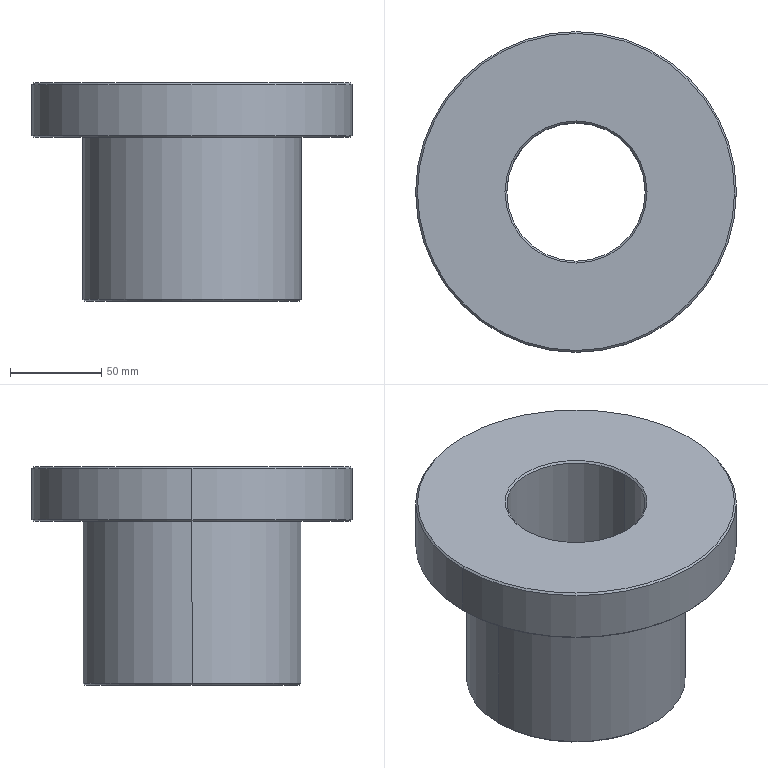Part | Creo | features DATUM PLANE 3, CURVE 2, PROTRUSION 2, CHAMFER 1, COORDINATE SYSTEM 1 | 1 solid | 19 faces | box 176 x 176 x 120 mm | volume 1202377 mm3 | cone 10 | cylinder 6 | plane 3 | commonest cylinder face diameters 76 x2 120 x2 176 x2
STEP:
#1=CARTESIAN_POINT('',(0.,0.,0.));
#2=DIRECTION('',(0.,0.,1.));
#3=DIRECTION('',(1.,0.,0.));
#4=AXIS2_PLACEMENT_3D('',#1,#2,#3);
#5=CARTESIAN_POINT('',(59.,0.,0.));
#6=VERTEX_POINT('',#5);
#7=CARTESIAN_POINT('',(-59.,0.,0.));
#8=VERTEX_POINT('',#7);
#9=CARTESIAN_POINT('',(0.,0.,0.));
#10=DIRECTION('',(0.,0.,-1.));
#11=DIRECTION('',(1.,0.,0.));
#12=AXIS2_PLACEMENT_3D('',#9,#10,#11);
#13=CIRCLE('',#12,59.);
#14=EDGE_CURVE('',#6,#8,#13,.T.);
#15=ORIENTED_EDGE('',*,*,#14,.F.);
#16=CARTESIAN_POINT('',(0.,0.,0.));
#17=DIRECTION('',(0.,0.,-1.));
#18=DIRECTION('',(-1.,0.,0.));
#19=AXIS2_PLACEMENT_3D('',#16,#17,#18);
#20=CIRCLE('',#19,59.);
#21=EDGE_CURVE('',#8,#6,#20,.T.);
#22=ORIENTED_EDGE('',*,*,#21,.F.);
#23=EDGE_LOOP('',(#15,#22));
#24=FACE_OUTER_BOUND('',#23,.F.);
#25=CARTESIAN_POINT('',(39.,0.,0.));
#26=VERTEX_POINT('',#25);
#27=CARTESIAN_POINT('',(-39.,0.,0.));
#28=VERTEX_POINT('',#27);
#29=CARTESIAN_POINT('',(0.,0.,0.));
#30=DIRECTION('',(0.,0.,1.));
#31=DIRECTION('',(1.,0.,0.));
#32=AXIS2_PLACEMENT_3D('',#29,#30,#31);
#33=CIRCLE('',#32,39.);
#34=EDGE_CURVE('',#26,#28,#33,.T.);
#35=ORIENTED_EDGE('',*,*,#34,.F.);
#36=CARTESIAN_POINT('',(0.,0.,0.));
#37=DIRECTION('',(0.,0.,1.));
#38=DIRECTION('',(-1.,0.,0.));
#39=AXIS2_PLACEMENT_3D('',#36,#37,#38);
#40=CIRCLE('',#39,39.);
#41=EDGE_CURVE('',#28,#26,#40,.T.);
#42=ORIENTED_EDGE('',*,*,#41,.F.);
#43=EDGE_LOOP('',(#35,#42));
#44=FACE_BOUND('',#43,.F.);
#45=CARTESIAN_POINT('',(0.,0.,0.));
#46=DIRECTION('',(0.,0.,1.));
#47=DIRECTION('',(1.,0.,0.));
#48=AXIS2_PLACEMENT_3D('',#45,#46,#47);
#49=PLANE('',#48);
#50=ADVANCED_FACE('',(#24,#44),#49,.F.);
#51=ORIENTED_EDGE('',*,*,#14,.T.);
#52=CARTESIAN_POINT('',(-60.,0.,1.));
#53=VERTEX_POINT('',#52);
#54=CARTESIAN_POINT('',(-59.,-0.000000017,-0.000000001));
#55=DIRECTION('',(-0.7071,0.000000003,0.7071));
#56=VECTOR('',#55,1.414);
#57=LINE('',#54,#56);
#58=EDGE_CURVE('',#8,#53,#57,.T.);
#59=ORIENTED_EDGE('',*,*,#58,.T.);
#60=CARTESIAN_POINT('',(60.,0.,1.));
#61=VERTEX_POINT('',#60);
#62=CARTESIAN_POINT('',(0.,0.,1.));
#63=DIRECTION('',(0.,0.,-1.));
#64=DIRECTION('',(1.,0.,0.));
#65=AXIS2_PLACEMENT_3D('',#62,#63,#64);
#66=CIRCLE('',#65,60.);
#67=EDGE_CURVE('',#61,#53,#66,.T.);
#68=ORIENTED_EDGE('',*,*,#67,.F.);
#69=CARTESIAN_POINT('',(59.,0.000000017,-0.000000001));
#70=DIRECTION('',(0.7071,-0.000000003,0.7071));
#71=VECTOR('',#70,1.414);
#72=LINE('',#69,#71);
#73=EDGE_CURVE('',#6,#61,#72,.T.);
#74=ORIENTED_EDGE('',*,*,#73,.F.);
#75=EDGE_LOOP('',(#51,#59,#68,#74));
#76=FACE_OUTER_BOUND('',#75,.F.);
#77=CARTESIAN_POINT('',(0.,0.,0.5));
#78=DIRECTION('',(0.,0.,1.));
#79=DIRECTION('',(0.,-1.,0.));
#80=AXIS2_PLACEMENT_3D('',#77,#78,#79);
#81=CONICAL_SURFACE('',#80,59.5,45.);
#82=ADVANCED_FACE('',(#76),#81,.T.);
#83=ORIENTED_EDGE('',*,*,#21,.T.);
#84=ORIENTED_EDGE('',*,*,#73,.T.);
#85=CARTESIAN_POINT('',(0.,0.,1.));
#86=DIRECTION('',(0.,0.,-1.));
#87=DIRECTION('',(-1.,0.,0.));
#88=AXIS2_PLACEMENT_3D('',#85,#86,#87);
#89=CIRCLE('',#88,60.);
#90=EDGE_CURVE('',#53,#61,#89,.T.);
#91=ORIENTED_EDGE('',*,*,#90,.F.);
#92=ORIENTED_EDGE('',*,*,#58,.F.);
#93=EDGE_LOOP('',(#83,#84,#91,#92));
#94=FACE_OUTER_BOUND('',#93,.F.);
#95=CARTESIAN_POINT('',(0.,0.,0.5));
#96=DIRECTION('',(0.,0.,1.));
#97=DIRECTION('',(0.,-1.,0.));
#98=AXIS2_PLACEMENT_3D('',#95,#96,#97);
#99=CONICAL_SURFACE('',#98,59.5,45.);
#100=ADVANCED_FACE('',(#94),#99,.T.);
#101=ORIENTED_EDGE('',*,*,#90,.T.);
#102=CARTESIAN_POINT('',(60.,0.,90.));
#103=VERTEX_POINT('',#102);
#104=CARTESIAN_POINT('',(60.,0.000000013,1.));
#105=DIRECTION('',(0.,0.,1.));
#106=VECTOR('',#105,89.);
#107=LINE('',#104,#106);
#108=EDGE_CURVE('',#61,#103,#107,.T.);
#109=ORIENTED_EDGE('',*,*,#108,.T.);
#110=CARTESIAN_POINT('',(-60.,0.,90.));
#111=VERTEX_POINT('',#110);
#112=CARTESIAN_POINT('',(0.,0.,90.));
#113=DIRECTION('',(0.,0.,1.));
#114=DIRECTION('',(1.,0.,0.));
#115=AXIS2_PLACEMENT_3D('',#112,#113,#114);
#116=CIRCLE('',#115,60.);
#117=EDGE_CURVE('',#103,#111,#116,.T.);
#118=ORIENTED_EDGE('',*,*,#117,.T.);
#119=CARTESIAN_POINT('',(-60.,-0.000000013,1.));
#120=DIRECTION('',(0.,0.,1.));
#121=VECTOR('',#120,89.);
#122=LINE('',#119,#121);
#123=EDGE_CURVE('',#53,#111,#122,.T.);
#124=ORIENTED_EDGE('',*,*,#123,.F.);
#125=EDGE_LOOP('',(#101,#109,#118,#124));
#126=FACE_OUTER_BOUND('',#125,.F.);
#127=CARTESIAN_POINT('',(0.,0.,0.));
#128=DIRECTION('',(0.,0.,1.));
#129=DIRECTION('',(1.,0.,0.));
#130=AXIS2_PLACEMENT_3D('',#127,#128,#129);
#131=CYLINDRICAL_SURFACE('',#130,60.);
#132=ADVANCED_FACE('',(#126),#131,.T.);
#133=ORIENTED_EDGE('',*,*,#67,.T.);
#134=ORIENTED_EDGE('',*,*,#123,.T.);
#135=CARTESIAN_POINT('',(0.,0.,90.));
#136=DIRECTION('',(0.,0.,1.));
#137=DIRECTION('',(-1.,0.,0.));
#138=AXIS2_PLACEMENT_3D('',#135,#136,#137);
#139=CIRCLE('',#138,60.);
#140=EDGE_CURVE('',#111,#103,#139,.T.);
#141=ORIENTED_EDGE('',*,*,#140,.T.);
#142=ORIENTED_EDGE('',*,*,#108,.F.);
#143=EDGE_LOOP('',(#133,#134,#141,#142));
#144=FACE_OUTER_BOUND('',#143,.F.);
#145=CARTESIAN_POINT('',(0.,0.,0.));
#146=DIRECTION('',(0.,0.,1.));
#147=DIRECTION('',(1.,0.,0.));
#148=AXIS2_PLACEMENT_3D('',#145,#146,#147);
#149=CYLINDRICAL_SURFACE('',#148,60.);
#150=ADVANCED_FACE('',(#144),#149,.T.);
#151=CARTESIAN_POINT('',(87.,0.,90.));
#152=VERTEX_POINT('',#151);
#153=CARTESIAN_POINT('',(-87.,0.,90.));
#154=VERTEX_POINT('',#153);
#155=CARTESIAN_POINT('',(0.,0.,90.));
#156=DIRECTION('',(0.,0.,-1.));
#157=DIRECTION('',(1.,0.,0.));
#158=AXIS2_PLACEMENT_3D('',#155,#156,#157);
#159=CIRCLE('',#158,87.);
#160=EDGE_CURVE('',#152,#154,#159,.T.);
#161=ORIENTED_EDGE('',*,*,#160,.F.);
#162=CARTESIAN_POINT('',(0.,0.,90.));
#163=DIRECTION('',(0.,0.,-1.));
#164=DIRECTION('',(-1.,0.,0.));
#165=AXIS2_PLACEMENT_3D('',#162,#163,#164);
#166=CIRCLE('',#165,87.);
#167=EDGE_CURVE('',#154,#152,#166,.T.);
#168=ORIENTED_EDGE('',*,*,#167,.F.);
#169=EDGE_LOOP('',(#161,#168));
#170=FACE_OUTER_BOUND('',#169,.F.);
#171=ORIENTED_EDGE('',*,*,#117,.F.);
#172=ORIENTED_EDGE('',*,*,#140,.F.);
#173=EDGE_LOOP('',(#171,#172));
#174=FACE_BOUND('',#173,.F.);
#175=CARTESIAN_POINT('',(0.,0.,90.));
#176=DIRECTION('',(0.,0.,1.));
#177=DIRECTION('',(1.,0.,0.));
#178=AXIS2_PLACEMENT_3D('',#175,#176,#177);
#179=PLANE('',#178);
#180=ADVANCED_FACE('',(#170,#174),#179,.F.);
#181=ORIENTED_EDGE('',*,*,#160,.T.);
#182=CARTESIAN_POINT('',(-88.,0.,91.));
#183=VERTEX_POINT('',#182);
#184=CARTESIAN_POINT('',(-87.,-0.000000014,90.));
#185=DIRECTION('',(-0.7071,0.000000002,0.7071));
#186=VECTOR('',#185,1.414);
#187=LINE('',#184,#186);
#188=EDGE_CURVE('',#154,#183,#187,.T.);
#189=ORIENTED_EDGE('',*,*,#188,.T.);
#190=CARTESIAN_POINT('',(88.,0.,91.));
#191=VERTEX_POINT('',#190);
#192=CARTESIAN_POINT('',(0.,0.,91.));
#193=DIRECTION('',(0.,0.,-1.));
#194=DIRECTION('',(1.,0.,0.));
#195=AXIS2_PLACEMENT_3D('',#192,#193,#194);
#196=CIRCLE('',#195,88.);
#197=EDGE_CURVE('',#191,#183,#196,.T.);
#198=ORIENTED_EDGE('',*,*,#197,.F.);
#199=CARTESIAN_POINT('',(87.,0.000000014,90.));
#200=DIRECTION('',(0.7071,-0.000000002,0.7071));
#201=VECTOR('',#200,1.414);
#202=LINE('',#199,#201);
#203=EDGE_CURVE('',#152,#191,#202,.T.);
#204=ORIENTED_EDGE('',*,*,#203,.F.);
#205=EDGE_LOOP('',(#181,#189,#198,#204));
#206=FACE_OUTER_BOUND('',#205,.F.);
#207=CARTESIAN_POINT('',(0.,0.,90.5));
#208=DIRECTION('',(0.,0.,1.));
#209=DIRECTION('',(0.,-1.,0.));
#210=AXIS2_PLACEMENT_3D('',#207,#208,#209);
#211=CONICAL_SURFACE('',#210,87.5,45.);
#212=ADVANCED_FACE('',(#206),#211,.T.);
#213=ORIENTED_EDGE('',*,*,#167,.T.);
#214=ORIENTED_EDGE('',*,*,#203,.T.);
#215=CARTESIAN_POINT('',(0.,0.,91.));
#216=DIRECTION('',(0.,0.,-1.));
#217=DIRECTION('',(-1.,0.,0.));
#218=AXIS2_PLACEMENT_3D('',#215,#216,#217);
#219=CIRCLE('',#218,88.);
#220=EDGE_CURVE('',#183,#191,#219,.T.);
#221=ORIENTED_EDGE('',*,*,#220,.F.);
#222=ORIENTED_EDGE('',*,*,#188,.F.);
#223=EDGE_LOOP('',(#213,#214,#221,#222));
#224=FACE_OUTER_BOUND('',#223,.F.);
#225=CARTESIAN_POINT('',(0.,0.,90.5));
#226=DIRECTION('',(0.,0.,1.));
#227=DIRECTION('',(0.,-1.,0.));
#228=AXIS2_PLACEMENT_3D('',#225,#226,#227);
#229=CONICAL_SURFACE('',#228,87.5,45.);
#230=ADVANCED_FACE('',(#224),#229,.T.);
#231=CARTESIAN_POINT('',(88.,0.,119.));
#232=VERTEX_POINT('',#231);
#233=CARTESIAN_POINT('',(-88.,0.,119.));
#234=VERTEX_POINT('',#233);
#235=CARTESIAN_POINT('',(0.,0.,119.));
#236=DIRECTION('',(0.,0.,1.));
#237=DIRECTION('',(1.,0.,0.));
#238=AXIS2_PLACEMENT_3D('',#235,#236,#237);
#239=CIRCLE('',#238,88.);
#240=EDGE_CURVE('',#232,#234,#239,.T.);
#241=ORIENTED_EDGE('',*,*,#240,.T.);
#242=CARTESIAN_POINT('',(-88.,-0.000000011,91.));
#243=DIRECTION('',(0.,0.,1.));
#244=VECTOR('',#243,28.);
#245=LINE('',#242,#244);
#246=EDGE_CURVE('',#183,#234,#245,.T.);
#247=ORIENTED_EDGE('',*,*,#246,.F.);
#248=ORIENTED_EDGE('',*,*,#220,.T.);
#249=CARTESIAN_POINT('',(88.,0.000000011,91.));
#250=DIRECTION('',(0.,0.,1.));
#251=VECTOR('',#250,28.);
#252=LINE('',#249,#251);
#253=EDGE_CURVE('',#191,#232,#252,.T.);
#254=ORIENTED_EDGE('',*,*,#253,.T.);
#255=EDGE_LOOP('',(#241,#247,#248,#254));
#256=FACE_OUTER_BOUND('',#255,.F.);
#257=CARTESIAN_POINT('',(0.,0.,90.));
#258=DIRECTION('',(0.,0.,1.));
#259=DIRECTION('',(1.,0.,0.));
#260=AXIS2_PLACEMENT_3D('',#257,#258,#259);
#261=CYLINDRICAL_SURFACE('',#260,88.);
#262=ADVANCED_FACE('',(#256),#261,.T.);
#263=CARTESIAN_POINT('',(87.,0.,120.));
#264=VERTEX_POINT('',#263);
#265=CARTESIAN_POINT('',(-87.,0.,120.));
#266=VERTEX_POINT('',#265);
#267=CARTESIAN_POINT('',(0.,0.,120.));
#268=DIRECTION('',(0.,0.,1.));
#269=DIRECTION('',(1.,0.,0.));
#270=AXIS2_PLACEMENT_3D('',#267,#268,#269);
#271=CIRCLE('',#270,87.);
#272=EDGE_CURVE('',#264,#266,#271,.T.);
#273=ORIENTED_EDGE('',*,*,#272,.T.);
#274=CARTESIAN_POINT('',(-87.,-0.000000014,120.));
#275=DIRECTION('',(-0.7071,0.000000002,-0.7071));
#276=VECTOR('',#275,1.414);
#277=LINE('',#274,#276);
#278=EDGE_CURVE('',#266,#234,#277,.T.);
#279=ORIENTED_EDGE('',*,*,#278,.T.);
#280=ORIENTED_EDGE('',*,*,#240,.F.);
#281=CARTESIAN_POINT('',(87.,0.000000014,120.));
#282=DIRECTION('',(0.7071,-0.000000002,-0.7071));
#283=VECTOR('',#282,1.414);
#284=LINE('',#281,#283);
#285=EDGE_CURVE('',#264,#232,#284,.T.);
#286=ORIENTED_EDGE('',*,*,#285,.F.);
#287=EDGE_LOOP('',(#273,#279,#280,#286));
#288=FACE_OUTER_BOUND('',#287,.F.);
#289=CARTESIAN_POINT('',(0.,0.,119.5));
#290=DIRECTION('',(0.,0.,-1.));
#291=DIRECTION('',(0.,-1.,0.));
#292=AXIS2_PLACEMENT_3D('',#289,#290,#291);
#293=CONICAL_SURFACE('',#292,87.5,45.);
#294=ADVANCED_FACE('',(#288),#293,.T.);
#295=CARTESIAN_POINT('',(0.,0.,120.));
#296=DIRECTION('',(0.,0.,1.));
#297=DIRECTION('',(-1.,0.,0.));
#298=AXIS2_PLACEMENT_3D('',#295,#296,#297);
#299=CIRCLE('',#298,87.);
#300=EDGE_CURVE('',#266,#264,#299,.T.);
#301=ORIENTED_EDGE('',*,*,#300,.F.);
#302=ORIENTED_EDGE('',*,*,#272,.F.);
#303=EDGE_LOOP('',(#301,#302));
#304=FACE_OUTER_BOUND('',#303,.F.);
#305=CARTESIAN_POINT('',(39.,0.,120.));
#306=VERTEX_POINT('',#305);
#307=CARTESIAN_POINT('',(-39.,0.,120.));
#308=VERTEX_POINT('',#307);
#309=CARTESIAN_POINT('',(0.,0.,120.));
#310=DIRECTION('',(0.,0.,-1.));
#311=DIRECTION('',(1.,0.,0.));
#312=AXIS2_PLACEMENT_3D('',#309,#310,#311);
#313=CIRCLE('',#312,39.);
#314=EDGE_CURVE('',#306,#308,#313,.T.);
#315=ORIENTED_EDGE('',*,*,#314,.F.);
#316=CARTESIAN_POINT('',(0.,0.,120.));
#317=DIRECTION('',(0.,0.,-1.));
#318=DIRECTION('',(-1.,0.,0.));
#319=AXIS2_PLACEMENT_3D('',#316,#317,#318);
#320=CIRCLE('',#319,39.);
#321=EDGE_CURVE('',#308,#306,#320,.T.);
#322=ORIENTED_EDGE('',*,*,#321,.F.);
#323=EDGE_LOOP('',(#315,#322));
#324=FACE_BOUND('',#323,.F.);
#325=CARTESIAN_POINT('',(0.,0.,120.));
#326=DIRECTION('',(0.,0.,1.));
#327=DIRECTION('',(1.,0.,0.));
#328=AXIS2_PLACEMENT_3D('',#325,#326,#327);
#329=PLANE('',#328);
#330=ADVANCED_FACE('',(#304,#324),#329,.T.);
#331=ORIENTED_EDGE('',*,*,#300,.T.);
#332=ORIENTED_EDGE('',*,*,#285,.T.);
#333=CARTESIAN_POINT('',(0.,0.,119.));
#334=DIRECTION('',(0.,0.,1.));
#335=DIRECTION('',(-1.,0.,0.));
#336=AXIS2_PLACEMENT_3D('',#333,#334,#335);
#337=CIRCLE('',#336,88.);
#338=EDGE_CURVE('',#234,#232,#337,.T.);
#339=ORIENTED_EDGE('',*,*,#338,.F.);
#340=ORIENTED_EDGE('',*,*,#278,.F.);
#341=EDGE_LOOP('',(#331,#332,#339,#340));
#342=FACE_OUTER_BOUND('',#341,.F.);
#343=CARTESIAN_POINT('',(0.,0.,119.5));
#344=DIRECTION('',(0.,0.,-1.));
#345=DIRECTION('',(0.,-1.,0.));
#346=AXIS2_PLACEMENT_3D('',#343,#344,#345);
#347=CONICAL_SURFACE('',#346,87.5,45.);
#348=ADVANCED_FACE('',(#342),#347,.T.);
#349=ORIENTED_EDGE('',*,*,#338,.T.);
#350=ORIENTED_EDGE('',*,*,#253,.F.);
#351=ORIENTED_EDGE('',*,*,#197,.T.);
#352=ORIENTED_EDGE('',*,*,#246,.T.);
#353=EDGE_LOOP('',(#349,#350,#351,#352));
#354=FACE_OUTER_BOUND('',#353,.F.);
#355=CARTESIAN_POINT('',(0.,0.,90.));
#356=DIRECTION('',(0.,0.,1.));
#357=DIRECTION('',(1.,0.,0.));
#358=AXIS2_PLACEMENT_3D('',#355,#356,#357);
#359=CYLINDRICAL_SURFACE('',#358,88.);
#360=ADVANCED_FACE('',(#354),#359,.T.);
#361=ORIENTED_EDGE('',*,*,#314,.T.);
#362=CARTESIAN_POINT('',(-38.,0.,119.));
#363=VERTEX_POINT('',#362);
#364=CARTESIAN_POINT('',(-39.,-0.000000025,120.));
#365=DIRECTION('',(0.7071,0.000000005,-0.7071));
#366=VECTOR('',#365,1.414);
#367=LINE('',#364,#366);
#368=EDGE_CURVE('',#308,#363,#367,.T.);
#369=ORIENTED_EDGE('',*,*,#368,.T.);
#370=CARTESIAN_POINT('',(38.,0.,119.));
#371=VERTEX_POINT('',#370);
#372=CARTESIAN_POINT('',(0.,0.,119.));
#373=DIRECTION('',(0.,0.,-1.));
#374=DIRECTION('',(1.,0.,0.));
#375=AXIS2_PLACEMENT_3D('',#372,#373,#374);
#376=CIRCLE('',#375,38.);
#377=EDGE_CURVE('',#371,#363,#376,.T.);
#378=ORIENTED_EDGE('',*,*,#377,.F.);
#379=CARTESIAN_POINT('',(39.,0.000000025,120.));
#380=DIRECTION('',(-0.7071,-0.000000005,-0.7071));
#381=VECTOR('',#380,1.414);
#382=LINE('',#379,#381);
#383=EDGE_CURVE('',#306,#371,#382,.T.);
#384=ORIENTED_EDGE('',*,*,#383,.F.);
#385=EDGE_LOOP('',(#361,#369,#378,#384));
#386=FACE_OUTER_BOUND('',#385,.F.);
#387=CARTESIAN_POINT('',(0.,0.,119.5));
#388=DIRECTION('',(0.,0.,1.));
#389=DIRECTION('',(0.,-1.,0.));
#390=AXIS2_PLACEMENT_3D('',#387,#388,#389);
#391=CONICAL_SURFACE('',#390,38.5,45.);
#392=ADVANCED_FACE('',(#386),#391,.F.);
#393=ORIENTED_EDGE('',*,*,#321,.T.);
#394=ORIENTED_EDGE('',*,*,#383,.T.);
#395=CARTESIAN_POINT('',(0.,0.,119.));
#396=DIRECTION('',(0.,0.,-1.));
#397=DIRECTION('',(-1.,0.,0.));
#398=AXIS2_PLACEMENT_3D('',#395,#396,#397);
#399=CIRCLE('',#398,38.);
#400=EDGE_CURVE('',#363,#371,#399,.T.);
#401=ORIENTED_EDGE('',*,*,#400,.F.);
#402=ORIENTED_EDGE('',*,*,#368,.F.);
#403=EDGE_LOOP('',(#393,#394,#401,#402));
#404=FACE_OUTER_BOUND('',#403,.F.);
#405=CARTESIAN_POINT('',(0.,0.,119.5));
#406=DIRECTION('',(0.,0.,1.));
#407=DIRECTION('',(0.,-1.,0.));
#408=AXIS2_PLACEMENT_3D('',#405,#406,#407);
#409=CONICAL_SURFACE('',#408,38.5,45.);
#410=ADVANCED_FACE('',(#404),#409,.F.);
#411=ORIENTED_EDGE('',*,*,#400,.T.);
#412=CARTESIAN_POINT('',(38.,0.,1.));
#413=VERTEX_POINT('',#412);
#414=CARTESIAN_POINT('',(38.,0.000000018,119.));
#415=DIRECTION('',(0.,0.,-1.));
#416=VECTOR('',#415,118.);
#417=LINE('',#414,#416);
#418=EDGE_CURVE('',#371,#413,#417,.T.);
#419=ORIENTED_EDGE('',*,*,#418,.T.);
#420=CARTESIAN_POINT('',(-38.,0.,1.));
#421=VERTEX_POINT('',#420);
#422=CARTESIAN_POINT('',(0.,0.,1.));
#423=DIRECTION('',(0.,0.,1.));
#424=DIRECTION('',(1.,0.,0.));
#425=AXIS2_PLACEMENT_3D('',#422,#423,#424);
#426=CIRCLE('',#425,38.);
#427=EDGE_CURVE('',#413,#421,#426,.T.);
#428=ORIENTED_EDGE('',*,*,#427,.T.);
#429=CARTESIAN_POINT('',(-38.,-0.000000018,1.));
#430=DIRECTION('',(0.,0.,1.));
#431=VECTOR('',#430,118.);
#432=LINE('',#429,#431);
#433=EDGE_CURVE('',#421,#363,#432,.T.);
#434=ORIENTED_EDGE('',*,*,#433,.T.);
#435=EDGE_LOOP('',(#411,#419,#428,#434));
#436=FACE_OUTER_BOUND('',#435,.F.);
#437=CARTESIAN_POINT('',(0.,0.,0.));
#438=DIRECTION('',(0.,0.,1.));
#439=DIRECTION('',(1.,0.,0.));
#440=AXIS2_PLACEMENT_3D('',#437,#438,#439);
#441=CYLINDRICAL_SURFACE('',#440,38.);
#442=ADVANCED_FACE('',(#436),#441,.F.);
#443=ORIENTED_EDGE('',*,*,#377,.T.);
#444=ORIENTED_EDGE('',*,*,#433,.F.);
#445=CARTESIAN_POINT('',(0.,0.,1.));
#446=DIRECTION('',(0.,0.,1.));
#447=DIRECTION('',(-1.,0.,0.));
#448=AXIS2_PLACEMENT_3D('',#445,#446,#447);
#449=CIRCLE('',#448,38.);
#450=EDGE_CURVE('',#421,#413,#449,.T.);
#451=ORIENTED_EDGE('',*,*,#450,.T.);
#452=ORIENTED_EDGE('',*,*,#418,.F.);
#453=EDGE_LOOP('',(#443,#444,#451,#452));
#454=FACE_OUTER_BOUND('',#453,.F.);
#455=CARTESIAN_POINT('',(0.,0.,0.));
#456=DIRECTION('',(0.,0.,1.));
#457=DIRECTION('',(1.,0.,0.));
#458=AXIS2_PLACEMENT_3D('',#455,#456,#457);
#459=CYLINDRICAL_SURFACE('',#458,38.);
#460=ADVANCED_FACE('',(#454),#459,.F.);
#461=ORIENTED_EDGE('',*,*,#41,.T.);
#462=CARTESIAN_POINT('',(39.,0.000000025,0.000000003));
#463=DIRECTION('',(-0.7071,-0.000000005,0.7071));
#464=VECTOR('',#463,1.414);
#465=LINE('',#462,#464);
#466=EDGE_CURVE('',#26,#413,#465,.T.);
#467=ORIENTED_EDGE('',*,*,#466,.T.);
#468=ORIENTED_EDGE('',*,*,#450,.F.);
#469=CARTESIAN_POINT('',(-39.,-0.000000025,0.000000003));
#470=DIRECTION('',(0.7071,0.000000005,0.7071));
#471=VECTOR('',#470,1.414);
#472=LINE('',#469,#471);
#473=EDGE_CURVE('',#28,#421,#472,.T.);
#474=ORIENTED_EDGE('',*,*,#473,.F.);
#475=EDGE_LOOP('',(#461,#467,#468,#474));
#476=FACE_OUTER_BOUND('',#475,.F.);
#477=CARTESIAN_POINT('',(0.,0.,0.5));
#478=DIRECTION('',(0.,0.,-1.));
#479=DIRECTION('',(0.,-1.,0.));
#480=AXIS2_PLACEMENT_3D('',#477,#478,#479);
#481=CONICAL_SURFACE('',#480,38.5,45.);
#482=ADVANCED_FACE('',(#476),#481,.F.);
#483=ORIENTED_EDGE('',*,*,#34,.T.);
#484=ORIENTED_EDGE('',*,*,#473,.T.);
#485=ORIENTED_EDGE('',*,*,#427,.F.);
#486=ORIENTED_EDGE('',*,*,#466,.F.);
#487=EDGE_LOOP('',(#483,#484,#485,#486));
#488=FACE_OUTER_BOUND('',#487,.F.);
#489=CARTESIAN_POINT('',(0.,0.,0.5));
#490=DIRECTION('',(0.,0.,-1.));
#491=DIRECTION('',(0.,-1.,0.));
#492=AXIS2_PLACEMENT_3D('',#489,#490,#491);
#493=CONICAL_SURFACE('',#492,38.5,45.);
#494=ADVANCED_FACE('',(#488),#493,.F.);
#495=CLOSED_SHELL('',(#50,#82,#100,#132,#150,#180,#212,#230,#262,#294,#330,#348,#360,#392,#410,#442,#460,#482,#494));
#496=MANIFOLD_SOLID_BREP('',#495);
#497=(LENGTH_UNIT()NAMED_UNIT(*)SI_UNIT(.MILLI.,.METRE.));
#498=UNCERTAINTY_MEASURE_WITH_UNIT(LENGTH_MEASURE(0.02763),#497,'','');
#499=(NAMED_UNIT(*)PLANE_ANGLE_UNIT()SI_UNIT($,.RADIAN.));
#500=PLANE_ANGLE_MEASURE_WITH_UNIT(PLANE_ANGLE_MEASURE(0.01745),#499);
#501=(CONVERSION_BASED_UNIT('DEGREE',#500)NAMED_UNIT(*)PLANE_ANGLE_UNIT());
#502=(NAMED_UNIT(*)SI_UNIT($,.STERADIAN.)SOLID_ANGLE_UNIT());
#503=(GEOMETRIC_REPRESENTATION_CONTEXT(3)GLOBAL_UNCERTAINTY_ASSIGNED_CONTEXT((#498))GLOBAL_UNIT_ASSIGNED_CONTEXT((#497,#501,#502))REPRESENTATION_CONTEXT('',''));
#504=ADVANCED_BREP_SHAPE_REPRESENTATION('',(#4,#496),#503);